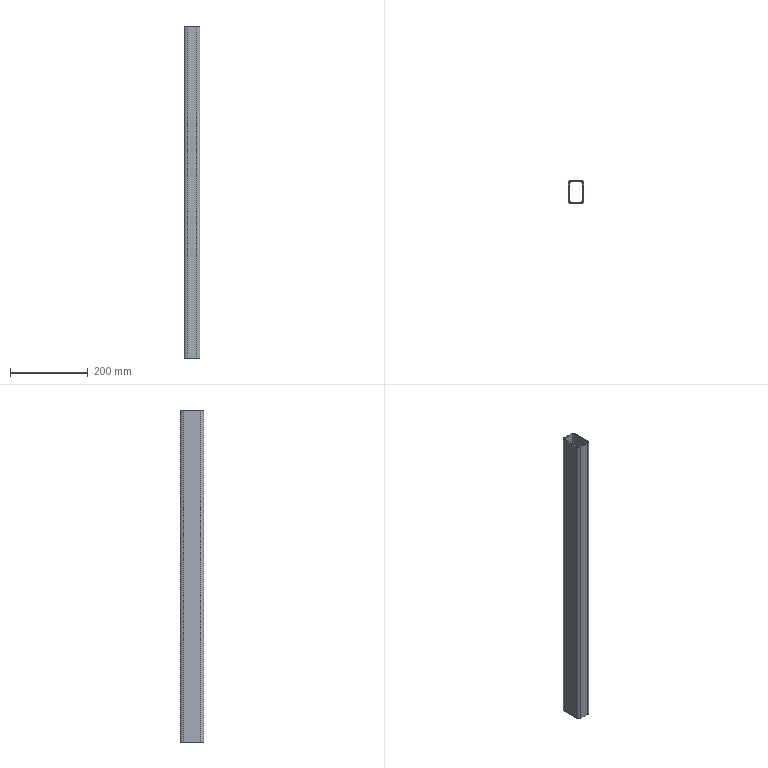Part | SolidWorks | features BaseBody 1 | 1 solid | 18 faces | box 40 x 60 x 852 mm | volume 454199 mm3 | plane 10 | cylinder 8 | commonest cylinder face diameters 9 x4 15 x4
STEP:
#1=CARTESIAN_POINT('',(17.,22.5,0.));
#2=VERTEX_POINT('',#1);
#3=CARTESIAN_POINT('',(17.,22.5,852.));
#4=VERTEX_POINT('',#3);
#5=CARTESIAN_POINT('',(17.,22.5,0.));
#6=DIRECTION('',(0.,0.,1.));
#7=VECTOR('',#6,1000.);
#8=LINE('',#5,#7);
#9=EDGE_CURVE('',#2,#4,#8,.T.);
#10=ORIENTED_EDGE('',*,*,#9,.F.);
#11=CARTESIAN_POINT('',(17.,-22.5,0.));
#12=VERTEX_POINT('',#11);
#13=CARTESIAN_POINT('',(17.,22.5,0.));
#14=DIRECTION('',(0.,1.,0.));
#15=VECTOR('',#14,1000.);
#16=LINE('',#13,#15);
#17=EDGE_CURVE('',#12,#2,#16,.T.);
#18=ORIENTED_EDGE('',*,*,#17,.F.);
#19=CARTESIAN_POINT('',(17.,-22.5,852.));
#20=VERTEX_POINT('',#19);
#21=CARTESIAN_POINT('',(17.,-22.5,0.));
#22=DIRECTION('',(0.,0.,-1.));
#23=VECTOR('',#22,1000.);
#24=LINE('',#21,#23);
#25=EDGE_CURVE('',#20,#12,#24,.T.);
#26=ORIENTED_EDGE('',*,*,#25,.F.);
#27=CARTESIAN_POINT('',(17.,22.5,852.));
#28=DIRECTION('',(0.,-1.,0.));
#29=VECTOR('',#28,1000.);
#30=LINE('',#27,#29);
#31=EDGE_CURVE('',#4,#20,#30,.T.);
#32=ORIENTED_EDGE('',*,*,#31,.F.);
#33=EDGE_LOOP('',(#10,#18,#26,#32));
#34=FACE_OUTER_BOUND('',#33,.T.);
#35=CARTESIAN_POINT('',(17.,22.5,0.));
#36=DIRECTION('',(1.,0.,0.));
#37=DIRECTION('',(0.,1.,0.));
#38=AXIS2_PLACEMENT_3D('',#35,#36,#37);
#39=PLANE('',#38);
#40=ADVANCED_FACE('',(#34),#39,.F.);
#41=CARTESIAN_POINT('',(-17.,-22.5,852.));
#42=VERTEX_POINT('',#41);
#43=CARTESIAN_POINT('',(-17.,22.5,852.));
#44=VERTEX_POINT('',#43);
#45=CARTESIAN_POINT('',(-17.,0.,852.));
#46=DIRECTION('',(0.,1.,0.));
#47=VECTOR('',#46,1000.);
#48=LINE('',#45,#47);
#49=EDGE_CURVE('',#42,#44,#48,.T.);
#50=ORIENTED_EDGE('',*,*,#49,.T.);
#51=CARTESIAN_POINT('',(-12.5,27.,852.));
#52=VERTEX_POINT('',#51);
#53=CARTESIAN_POINT('',(-12.5,22.5,852.));
#54=DIRECTION('',(0.,0.,-1.));
#55=DIRECTION('',(1.,0.,0.));
#56=AXIS2_PLACEMENT_3D('',#53,#54,#55);
#57=CIRCLE('',#56,4.5);
#58=EDGE_CURVE('',#44,#52,#57,.T.);
#59=ORIENTED_EDGE('',*,*,#58,.T.);
#60=CARTESIAN_POINT('',(12.5,27.,852.));
#61=VERTEX_POINT('',#60);
#62=CARTESIAN_POINT('',(0.,27.,852.));
#63=DIRECTION('',(1.,0.,0.));
#64=VECTOR('',#63,1000.);
#65=LINE('',#62,#64);
#66=EDGE_CURVE('',#52,#61,#65,.T.);
#67=ORIENTED_EDGE('',*,*,#66,.T.);
#68=CARTESIAN_POINT('',(12.5,22.5,852.));
#69=DIRECTION('',(0.,0.,-1.));
#70=DIRECTION('',(1.,0.,0.));
#71=AXIS2_PLACEMENT_3D('',#68,#69,#70);
#72=CIRCLE('',#71,4.5);
#73=EDGE_CURVE('',#61,#4,#72,.T.);
#74=ORIENTED_EDGE('',*,*,#73,.T.);
#75=ORIENTED_EDGE('',*,*,#31,.T.);
#76=CARTESIAN_POINT('',(12.5,-27.,852.));
#77=VERTEX_POINT('',#76);
#78=CARTESIAN_POINT('',(12.5,-22.5,852.));
#79=DIRECTION('',(0.,0.,-1.));
#80=DIRECTION('',(1.,0.,0.));
#81=AXIS2_PLACEMENT_3D('',#78,#79,#80);
#82=CIRCLE('',#81,4.5);
#83=EDGE_CURVE('',#20,#77,#82,.T.);
#84=ORIENTED_EDGE('',*,*,#83,.T.);
#85=CARTESIAN_POINT('',(-12.5,-27.,852.));
#86=VERTEX_POINT('',#85);
#87=CARTESIAN_POINT('',(0.,-27.,852.));
#88=DIRECTION('',(-1.,0.,0.));
#89=VECTOR('',#88,1000.);
#90=LINE('',#87,#89);
#91=EDGE_CURVE('',#77,#86,#90,.T.);
#92=ORIENTED_EDGE('',*,*,#91,.T.);
#93=CARTESIAN_POINT('',(-12.5,-22.5,852.));
#94=DIRECTION('',(0.,0.,-1.));
#95=DIRECTION('',(1.,0.,0.));
#96=AXIS2_PLACEMENT_3D('',#93,#94,#95);
#97=CIRCLE('',#96,4.5);
#98=EDGE_CURVE('',#86,#42,#97,.T.);
#99=ORIENTED_EDGE('',*,*,#98,.T.);
#100=EDGE_LOOP('',(#50,#59,#67,#74,#75,#84,#92,#99));
#101=FACE_BOUND('',#100,.T.);
#102=CARTESIAN_POINT('',(12.5,30.,852.));
#103=VERTEX_POINT('',#102);
#104=CARTESIAN_POINT('',(-12.5,30.,852.));
#105=VERTEX_POINT('',#104);
#106=CARTESIAN_POINT('',(0.,30.,852.));
#107=DIRECTION('',(-1.,0.,0.));
#108=VECTOR('',#107,1000.);
#109=LINE('',#106,#108);
#110=EDGE_CURVE('',#103,#105,#109,.T.);
#111=ORIENTED_EDGE('',*,*,#110,.T.);
#112=CARTESIAN_POINT('',(-20.,22.5,852.));
#113=VERTEX_POINT('',#112);
#114=CARTESIAN_POINT('',(-12.5,22.5,852.));
#115=DIRECTION('',(0.,0.,1.));
#116=DIRECTION('',(1.,0.,0.));
#117=AXIS2_PLACEMENT_3D('',#114,#115,#116);
#118=CIRCLE('',#117,7.5);
#119=EDGE_CURVE('',#105,#113,#118,.T.);
#120=ORIENTED_EDGE('',*,*,#119,.T.);
#121=CARTESIAN_POINT('',(-20.,-22.5,852.));
#122=VERTEX_POINT('',#121);
#123=CARTESIAN_POINT('',(-20.,0.,852.));
#124=DIRECTION('',(0.,-1.,0.));
#125=VECTOR('',#124,1000.);
#126=LINE('',#123,#125);
#127=EDGE_CURVE('',#113,#122,#126,.T.);
#128=ORIENTED_EDGE('',*,*,#127,.T.);
#129=CARTESIAN_POINT('',(-12.5,-30.,852.));
#130=VERTEX_POINT('',#129);
#131=CARTESIAN_POINT('',(-12.5,-22.5,852.));
#132=DIRECTION('',(0.,0.,1.));
#133=DIRECTION('',(1.,0.,0.));
#134=AXIS2_PLACEMENT_3D('',#131,#132,#133);
#135=CIRCLE('',#134,7.5);
#136=EDGE_CURVE('',#122,#130,#135,.T.);
#137=ORIENTED_EDGE('',*,*,#136,.T.);
#138=CARTESIAN_POINT('',(12.5,-30.,852.));
#139=VERTEX_POINT('',#138);
#140=CARTESIAN_POINT('',(0.,-30.,852.));
#141=DIRECTION('',(1.,0.,0.));
#142=VECTOR('',#141,1000.);
#143=LINE('',#140,#142);
#144=EDGE_CURVE('',#130,#139,#143,.T.);
#145=ORIENTED_EDGE('',*,*,#144,.T.);
#146=CARTESIAN_POINT('',(20.,-22.5,852.));
#147=VERTEX_POINT('',#146);
#148=CARTESIAN_POINT('',(12.5,-22.5,852.));
#149=DIRECTION('',(0.,0.,1.));
#150=DIRECTION('',(1.,0.,0.));
#151=AXIS2_PLACEMENT_3D('',#148,#149,#150);
#152=CIRCLE('',#151,7.5);
#153=EDGE_CURVE('',#139,#147,#152,.T.);
#154=ORIENTED_EDGE('',*,*,#153,.T.);
#155=CARTESIAN_POINT('',(20.,22.5,852.));
#156=VERTEX_POINT('',#155);
#157=CARTESIAN_POINT('',(20.,0.,852.));
#158=DIRECTION('',(0.,1.,0.));
#159=VECTOR('',#158,1000.);
#160=LINE('',#157,#159);
#161=EDGE_CURVE('',#147,#156,#160,.T.);
#162=ORIENTED_EDGE('',*,*,#161,.T.);
#163=CARTESIAN_POINT('',(12.5,22.5,852.));
#164=DIRECTION('',(0.,0.,1.));
#165=DIRECTION('',(1.,0.,0.));
#166=AXIS2_PLACEMENT_3D('',#163,#164,#165);
#167=CIRCLE('',#166,7.5);
#168=EDGE_CURVE('',#156,#103,#167,.T.);
#169=ORIENTED_EDGE('',*,*,#168,.T.);
#170=EDGE_LOOP('',(#111,#120,#128,#137,#145,#154,#162,#169));
#171=FACE_OUTER_BOUND('',#170,.T.);
#172=CARTESIAN_POINT('',(0.,0.,852.));
#173=DIRECTION('',(0.,0.,1.));
#174=DIRECTION('',(1.,0.,0.));
#175=AXIS2_PLACEMENT_3D('',#172,#173,#174);
#176=PLANE('',#175);
#177=ADVANCED_FACE('',(#101,#171),#176,.T.);
#178=CARTESIAN_POINT('',(12.5,27.,0.));
#179=VERTEX_POINT('',#178);
#180=CARTESIAN_POINT('',(12.5,27.,0.));
#181=DIRECTION('',(0.,0.,1.));
#182=VECTOR('',#181,1000.);
#183=LINE('',#180,#182);
#184=EDGE_CURVE('',#179,#61,#183,.T.);
#185=ORIENTED_EDGE('',*,*,#184,.F.);
#186=CARTESIAN_POINT('',(12.5,22.5,0.));
#187=DIRECTION('',(0.,0.,1.));
#188=DIRECTION('',(1.,0.,0.));
#189=AXIS2_PLACEMENT_3D('',#186,#187,#188);
#190=CIRCLE('',#189,4.5);
#191=EDGE_CURVE('',#2,#179,#190,.T.);
#192=ORIENTED_EDGE('',*,*,#191,.F.);
#193=ORIENTED_EDGE('',*,*,#9,.T.);
#194=ORIENTED_EDGE('',*,*,#73,.F.);
#195=EDGE_LOOP('',(#185,#192,#193,#194));
#196=FACE_OUTER_BOUND('',#195,.T.);
#197=CARTESIAN_POINT('',(12.5,22.5,0.));
#198=DIRECTION('',(0.,0.,1.));
#199=DIRECTION('',(1.,0.,0.));
#200=AXIS2_PLACEMENT_3D('',#197,#198,#199);
#201=CYLINDRICAL_SURFACE('',#200,4.5);
#202=ADVANCED_FACE('',(#196),#201,.F.);
#203=CARTESIAN_POINT('',(-17.,22.5,0.));
#204=VERTEX_POINT('',#203);
#205=CARTESIAN_POINT('',(-12.5,27.,0.));
#206=VERTEX_POINT('',#205);
#207=CARTESIAN_POINT('',(-12.5,22.5,0.));
#208=DIRECTION('',(0.,0.,-1.));
#209=DIRECTION('',(1.,0.,0.));
#210=AXIS2_PLACEMENT_3D('',#207,#208,#209);
#211=CIRCLE('',#210,4.5);
#212=EDGE_CURVE('',#204,#206,#211,.T.);
#213=ORIENTED_EDGE('',*,*,#212,.F.);
#214=CARTESIAN_POINT('',(-17.,-22.5,0.));
#215=VERTEX_POINT('',#214);
#216=CARTESIAN_POINT('',(-17.,0.,0.));
#217=DIRECTION('',(0.,1.,0.));
#218=VECTOR('',#217,1000.);
#219=LINE('',#216,#218);
#220=EDGE_CURVE('',#215,#204,#219,.T.);
#221=ORIENTED_EDGE('',*,*,#220,.F.);
#222=CARTESIAN_POINT('',(-12.5,-27.,0.));
#223=VERTEX_POINT('',#222);
#224=CARTESIAN_POINT('',(-12.5,-22.5,0.));
#225=DIRECTION('',(0.,0.,-1.));
#226=DIRECTION('',(1.,0.,0.));
#227=AXIS2_PLACEMENT_3D('',#224,#225,#226);
#228=CIRCLE('',#227,4.5);
#229=EDGE_CURVE('',#223,#215,#228,.T.);
#230=ORIENTED_EDGE('',*,*,#229,.F.);
#231=CARTESIAN_POINT('',(12.5,-27.,0.));
#232=VERTEX_POINT('',#231);
#233=CARTESIAN_POINT('',(0.,-27.,0.));
#234=DIRECTION('',(-1.,0.,0.));
#235=VECTOR('',#234,1000.);
#236=LINE('',#233,#235);
#237=EDGE_CURVE('',#232,#223,#236,.T.);
#238=ORIENTED_EDGE('',*,*,#237,.F.);
#239=CARTESIAN_POINT('',(12.5,-22.5,0.));
#240=DIRECTION('',(0.,0.,-1.));
#241=DIRECTION('',(1.,0.,0.));
#242=AXIS2_PLACEMENT_3D('',#239,#240,#241);
#243=CIRCLE('',#242,4.5);
#244=EDGE_CURVE('',#12,#232,#243,.T.);
#245=ORIENTED_EDGE('',*,*,#244,.F.);
#246=ORIENTED_EDGE('',*,*,#17,.T.);
#247=ORIENTED_EDGE('',*,*,#191,.T.);
#248=CARTESIAN_POINT('',(0.,27.,0.));
#249=DIRECTION('',(1.,0.,0.));
#250=VECTOR('',#249,1000.);
#251=LINE('',#248,#250);
#252=EDGE_CURVE('',#206,#179,#251,.T.);
#253=ORIENTED_EDGE('',*,*,#252,.F.);
#254=EDGE_LOOP('',(#213,#221,#230,#238,#245,#246,#247,#253));
#255=FACE_BOUND('',#254,.T.);
#256=CARTESIAN_POINT('',(-12.5,30.,0.));
#257=VERTEX_POINT('',#256);
#258=CARTESIAN_POINT('',(-20.,22.5,0.));
#259=VERTEX_POINT('',#258);
#260=CARTESIAN_POINT('',(-12.5,22.5,0.));
#261=DIRECTION('',(0.,0.,1.));
#262=DIRECTION('',(1.,0.,0.));
#263=AXIS2_PLACEMENT_3D('',#260,#261,#262);
#264=CIRCLE('',#263,7.5);
#265=EDGE_CURVE('',#257,#259,#264,.T.);
#266=ORIENTED_EDGE('',*,*,#265,.F.);
#267=CARTESIAN_POINT('',(12.5,30.,0.));
#268=VERTEX_POINT('',#267);
#269=CARTESIAN_POINT('',(0.,30.,0.));
#270=DIRECTION('',(-1.,0.,0.));
#271=VECTOR('',#270,1000.);
#272=LINE('',#269,#271);
#273=EDGE_CURVE('',#268,#257,#272,.T.);
#274=ORIENTED_EDGE('',*,*,#273,.F.);
#275=CARTESIAN_POINT('',(20.,22.5,0.));
#276=VERTEX_POINT('',#275);
#277=CARTESIAN_POINT('',(12.5,22.5,0.));
#278=DIRECTION('',(0.,0.,1.));
#279=DIRECTION('',(1.,0.,0.));
#280=AXIS2_PLACEMENT_3D('',#277,#278,#279);
#281=CIRCLE('',#280,7.5);
#282=EDGE_CURVE('',#276,#268,#281,.T.);
#283=ORIENTED_EDGE('',*,*,#282,.F.);
#284=CARTESIAN_POINT('',(20.,-22.5,0.));
#285=VERTEX_POINT('',#284);
#286=CARTESIAN_POINT('',(20.,0.,0.));
#287=DIRECTION('',(0.,1.,0.));
#288=VECTOR('',#287,1000.);
#289=LINE('',#286,#288);
#290=EDGE_CURVE('',#285,#276,#289,.T.);
#291=ORIENTED_EDGE('',*,*,#290,.F.);
#292=CARTESIAN_POINT('',(12.5,-30.,0.));
#293=VERTEX_POINT('',#292);
#294=CARTESIAN_POINT('',(12.5,-22.5,0.));
#295=DIRECTION('',(0.,0.,1.));
#296=DIRECTION('',(1.,0.,0.));
#297=AXIS2_PLACEMENT_3D('',#294,#295,#296);
#298=CIRCLE('',#297,7.5);
#299=EDGE_CURVE('',#293,#285,#298,.T.);
#300=ORIENTED_EDGE('',*,*,#299,.F.);
#301=CARTESIAN_POINT('',(-12.5,-30.,0.));
#302=VERTEX_POINT('',#301);
#303=CARTESIAN_POINT('',(0.,-30.,0.));
#304=DIRECTION('',(1.,0.,0.));
#305=VECTOR('',#304,1000.);
#306=LINE('',#303,#305);
#307=EDGE_CURVE('',#302,#293,#306,.T.);
#308=ORIENTED_EDGE('',*,*,#307,.F.);
#309=CARTESIAN_POINT('',(-20.,-22.5,0.));
#310=VERTEX_POINT('',#309);
#311=CARTESIAN_POINT('',(-12.5,-22.5,0.));
#312=DIRECTION('',(0.,0.,1.));
#313=DIRECTION('',(1.,0.,0.));
#314=AXIS2_PLACEMENT_3D('',#311,#312,#313);
#315=CIRCLE('',#314,7.5);
#316=EDGE_CURVE('',#310,#302,#315,.T.);
#317=ORIENTED_EDGE('',*,*,#316,.F.);
#318=CARTESIAN_POINT('',(-20.,0.,0.));
#319=DIRECTION('',(0.,-1.,0.));
#320=VECTOR('',#319,1000.);
#321=LINE('',#318,#320);
#322=EDGE_CURVE('',#259,#310,#321,.T.);
#323=ORIENTED_EDGE('',*,*,#322,.F.);
#324=EDGE_LOOP('',(#266,#274,#283,#291,#300,#308,#317,#323));
#325=FACE_OUTER_BOUND('',#324,.T.);
#326=CARTESIAN_POINT('',(0.,0.,0.));
#327=DIRECTION('',(0.,0.,1.));
#328=DIRECTION('',(1.,0.,0.));
#329=AXIS2_PLACEMENT_3D('',#326,#327,#328);
#330=PLANE('',#329);
#331=ADVANCED_FACE('',(#255,#325),#330,.F.);
#332=ORIENTED_EDGE('',*,*,#25,.T.);
#333=ORIENTED_EDGE('',*,*,#244,.T.);
#334=CARTESIAN_POINT('',(12.5,-27.,0.));
#335=DIRECTION('',(0.,0.,-1.));
#336=VECTOR('',#335,1000.);
#337=LINE('',#334,#336);
#338=EDGE_CURVE('',#77,#232,#337,.T.);
#339=ORIENTED_EDGE('',*,*,#338,.F.);
#340=ORIENTED_EDGE('',*,*,#83,.F.);
#341=EDGE_LOOP('',(#332,#333,#339,#340));
#342=FACE_OUTER_BOUND('',#341,.T.);
#343=CARTESIAN_POINT('',(12.5,-22.5,0.));
#344=DIRECTION('',(0.,0.,1.));
#345=DIRECTION('',(1.,0.,0.));
#346=AXIS2_PLACEMENT_3D('',#343,#344,#345);
#347=CYLINDRICAL_SURFACE('',#346,4.5);
#348=ADVANCED_FACE('',(#342),#347,.F.);
#349=CARTESIAN_POINT('',(-17.,22.5,0.));
#350=DIRECTION('',(0.,0.,1.));
#351=VECTOR('',#350,1000.);
#352=LINE('',#349,#351);
#353=EDGE_CURVE('',#204,#44,#352,.T.);
#354=ORIENTED_EDGE('',*,*,#353,.F.);
#355=ORIENTED_EDGE('',*,*,#212,.T.);
#356=CARTESIAN_POINT('',(-12.5,27.,0.));
#357=DIRECTION('',(0.,0.,-1.));
#358=VECTOR('',#357,1000.);
#359=LINE('',#356,#358);
#360=EDGE_CURVE('',#52,#206,#359,.T.);
#361=ORIENTED_EDGE('',*,*,#360,.F.);
#362=ORIENTED_EDGE('',*,*,#58,.F.);
#363=EDGE_LOOP('',(#354,#355,#361,#362));
#364=FACE_OUTER_BOUND('',#363,.T.);
#365=CARTESIAN_POINT('',(-12.5,22.5,0.));
#366=DIRECTION('',(0.,0.,1.));
#367=DIRECTION('',(1.,0.,0.));
#368=AXIS2_PLACEMENT_3D('',#365,#366,#367);
#369=CYLINDRICAL_SURFACE('',#368,4.5);
#370=ADVANCED_FACE('',(#364),#369,.F.);
#371=CARTESIAN_POINT('',(-17.,-22.5,0.));
#372=DIRECTION('',(0.,0.,1.));
#373=VECTOR('',#372,1000.);
#374=LINE('',#371,#373);
#375=EDGE_CURVE('',#215,#42,#374,.T.);
#376=ORIENTED_EDGE('',*,*,#375,.F.);
#377=ORIENTED_EDGE('',*,*,#220,.T.);
#378=ORIENTED_EDGE('',*,*,#353,.T.);
#379=ORIENTED_EDGE('',*,*,#49,.F.);
#380=EDGE_LOOP('',(#376,#377,#378,#379));
#381=FACE_OUTER_BOUND('',#380,.T.);
#382=CARTESIAN_POINT('',(-17.,-22.5,0.));
#383=DIRECTION('',(-1.,0.,0.));
#384=DIRECTION('',(0.,-1.,0.));
#385=AXIS2_PLACEMENT_3D('',#382,#383,#384);
#386=PLANE('',#385);
#387=ADVANCED_FACE('',(#381),#386,.F.);
#388=CARTESIAN_POINT('',(-12.5,-27.,0.));
#389=DIRECTION('',(0.,0.,1.));
#390=VECTOR('',#389,1000.);
#391=LINE('',#388,#390);
#392=EDGE_CURVE('',#223,#86,#391,.T.);
#393=ORIENTED_EDGE('',*,*,#392,.F.);
#394=ORIENTED_EDGE('',*,*,#229,.T.);
#395=ORIENTED_EDGE('',*,*,#375,.T.);
#396=ORIENTED_EDGE('',*,*,#98,.F.);
#397=EDGE_LOOP('',(#393,#394,#395,#396));
#398=FACE_OUTER_BOUND('',#397,.T.);
#399=CARTESIAN_POINT('',(-12.5,-22.5,0.));
#400=DIRECTION('',(0.,0.,1.));
#401=DIRECTION('',(1.,0.,0.));
#402=AXIS2_PLACEMENT_3D('',#399,#400,#401);
#403=CYLINDRICAL_SURFACE('',#402,4.5);
#404=ADVANCED_FACE('',(#398),#403,.F.);
#405=ORIENTED_EDGE('',*,*,#338,.T.);
#406=ORIENTED_EDGE('',*,*,#237,.T.);
#407=ORIENTED_EDGE('',*,*,#392,.T.);
#408=ORIENTED_EDGE('',*,*,#91,.F.);
#409=EDGE_LOOP('',(#405,#406,#407,#408));
#410=FACE_OUTER_BOUND('',#409,.T.);
#411=CARTESIAN_POINT('',(12.5,-27.,0.));
#412=DIRECTION('',(0.,-1.,0.));
#413=DIRECTION('',(1.,0.,0.));
#414=AXIS2_PLACEMENT_3D('',#411,#412,#413);
#415=PLANE('',#414);
#416=ADVANCED_FACE('',(#410),#415,.F.);
#417=ORIENTED_EDGE('',*,*,#360,.T.);
#418=ORIENTED_EDGE('',*,*,#252,.T.);
#419=ORIENTED_EDGE('',*,*,#184,.T.);
#420=ORIENTED_EDGE('',*,*,#66,.F.);
#421=EDGE_LOOP('',(#417,#418,#419,#420));
#422=FACE_OUTER_BOUND('',#421,.T.);
#423=CARTESIAN_POINT('',(-12.5,27.,0.));
#424=DIRECTION('',(0.,1.,0.));
#425=DIRECTION('',(-1.,0.,0.));
#426=AXIS2_PLACEMENT_3D('',#423,#424,#425);
#427=PLANE('',#426);
#428=ADVANCED_FACE('',(#422),#427,.F.);
#429=ORIENTED_EDGE('',*,*,#265,.T.);
#430=CARTESIAN_POINT('',(-20.,22.5,0.));
#431=DIRECTION('',(0.,0.,1.));
#432=VECTOR('',#431,1000.);
#433=LINE('',#430,#432);
#434=EDGE_CURVE('',#259,#113,#433,.T.);
#435=ORIENTED_EDGE('',*,*,#434,.T.);
#436=ORIENTED_EDGE('',*,*,#119,.F.);
#437=CARTESIAN_POINT('',(-12.5,30.,0.));
#438=DIRECTION('',(0.,0.,-1.));
#439=VECTOR('',#438,1000.);
#440=LINE('',#437,#439);
#441=EDGE_CURVE('',#105,#257,#440,.T.);
#442=ORIENTED_EDGE('',*,*,#441,.T.);
#443=EDGE_LOOP('',(#429,#435,#436,#442));
#444=FACE_OUTER_BOUND('',#443,.T.);
#445=CARTESIAN_POINT('',(-12.5,22.5,0.));
#446=DIRECTION('',(0.,0.,1.));
#447=DIRECTION('',(1.,0.,0.));
#448=AXIS2_PLACEMENT_3D('',#445,#446,#447);
#449=CYLINDRICAL_SURFACE('',#448,7.5);
#450=ADVANCED_FACE('',(#444),#449,.T.);
#451=ORIENTED_EDGE('',*,*,#273,.T.);
#452=ORIENTED_EDGE('',*,*,#441,.F.);
#453=ORIENTED_EDGE('',*,*,#110,.F.);
#454=CARTESIAN_POINT('',(12.5,30.,0.));
#455=DIRECTION('',(0.,0.,-1.));
#456=VECTOR('',#455,1000.);
#457=LINE('',#454,#456);
#458=EDGE_CURVE('',#103,#268,#457,.T.);
#459=ORIENTED_EDGE('',*,*,#458,.T.);
#460=EDGE_LOOP('',(#451,#452,#453,#459));
#461=FACE_OUTER_BOUND('',#460,.T.);
#462=CARTESIAN_POINT('',(-12.5,30.,0.));
#463=DIRECTION('',(0.,1.,0.));
#464=DIRECTION('',(0.,0.,1.));
#465=AXIS2_PLACEMENT_3D('',#462,#463,#464);
#466=PLANE('',#465);
#467=ADVANCED_FACE('',(#461),#466,.T.);
#468=ORIENTED_EDGE('',*,*,#282,.T.);
#469=ORIENTED_EDGE('',*,*,#458,.F.);
#470=ORIENTED_EDGE('',*,*,#168,.F.);
#471=CARTESIAN_POINT('',(20.,22.5,0.));
#472=DIRECTION('',(0.,0.,-1.));
#473=VECTOR('',#472,1000.);
#474=LINE('',#471,#473);
#475=EDGE_CURVE('',#156,#276,#474,.T.);
#476=ORIENTED_EDGE('',*,*,#475,.T.);
#477=EDGE_LOOP('',(#468,#469,#470,#476));
#478=FACE_OUTER_BOUND('',#477,.T.);
#479=CARTESIAN_POINT('',(12.5,22.5,0.));
#480=DIRECTION('',(0.,0.,1.));
#481=DIRECTION('',(1.,0.,0.));
#482=AXIS2_PLACEMENT_3D('',#479,#480,#481);
#483=CYLINDRICAL_SURFACE('',#482,7.5);
#484=ADVANCED_FACE('',(#478),#483,.T.);
#485=ORIENTED_EDGE('',*,*,#290,.T.);
#486=ORIENTED_EDGE('',*,*,#475,.F.);
#487=ORIENTED_EDGE('',*,*,#161,.F.);
#488=CARTESIAN_POINT('',(20.,-22.5,0.));
#489=DIRECTION('',(0.,0.,-1.));
#490=VECTOR('',#489,1000.);
#491=LINE('',#488,#490);
#492=EDGE_CURVE('',#147,#285,#491,.T.);
#493=ORIENTED_EDGE('',*,*,#492,.T.);
#494=EDGE_LOOP('',(#485,#486,#487,#493));
#495=FACE_OUTER_BOUND('',#494,.T.);
#496=CARTESIAN_POINT('',(20.,22.5,0.));
#497=DIRECTION('',(1.,0.,0.));
#498=DIRECTION('',(0.,0.,-1.));
#499=AXIS2_PLACEMENT_3D('',#496,#497,#498);
#500=PLANE('',#499);
#501=ADVANCED_FACE('',(#495),#500,.T.);
#502=ORIENTED_EDGE('',*,*,#299,.T.);
#503=ORIENTED_EDGE('',*,*,#492,.F.);
#504=ORIENTED_EDGE('',*,*,#153,.F.);
#505=CARTESIAN_POINT('',(12.5,-30.,0.));
#506=DIRECTION('',(0.,0.,-1.));
#507=VECTOR('',#506,1000.);
#508=LINE('',#505,#507);
#509=EDGE_CURVE('',#139,#293,#508,.T.);
#510=ORIENTED_EDGE('',*,*,#509,.T.);
#511=EDGE_LOOP('',(#502,#503,#504,#510));
#512=FACE_OUTER_BOUND('',#511,.T.);
#513=CARTESIAN_POINT('',(12.5,-22.5,0.));
#514=DIRECTION('',(0.,0.,1.));
#515=DIRECTION('',(1.,0.,0.));
#516=AXIS2_PLACEMENT_3D('',#513,#514,#515);
#517=CYLINDRICAL_SURFACE('',#516,7.5);
#518=ADVANCED_FACE('',(#512),#517,.T.);
#519=ORIENTED_EDGE('',*,*,#307,.T.);
#520=ORIENTED_EDGE('',*,*,#509,.F.);
#521=ORIENTED_EDGE('',*,*,#144,.F.);
#522=CARTESIAN_POINT('',(-12.5,-30.,0.));
#523=DIRECTION('',(0.,0.,-1.));
#524=VECTOR('',#523,1000.);
#525=LINE('',#522,#524);
#526=EDGE_CURVE('',#130,#302,#525,.T.);
#527=ORIENTED_EDGE('',*,*,#526,.T.);
#528=EDGE_LOOP('',(#519,#520,#521,#527));
#529=FACE_OUTER_BOUND('',#528,.T.);
#530=CARTESIAN_POINT('',(12.5,-30.,0.));
#531=DIRECTION('',(0.,-1.,0.));
#532=DIRECTION('',(1.,0.,0.));
#533=AXIS2_PLACEMENT_3D('',#530,#531,#532);
#534=PLANE('',#533);
#535=ADVANCED_FACE('',(#529),#534,.T.);
#536=ORIENTED_EDGE('',*,*,#316,.T.);
#537=ORIENTED_EDGE('',*,*,#526,.F.);
#538=ORIENTED_EDGE('',*,*,#136,.F.);
#539=CARTESIAN_POINT('',(-20.,-22.5,0.));
#540=DIRECTION('',(0.,0.,-1.));
#541=VECTOR('',#540,1000.);
#542=LINE('',#539,#541);
#543=EDGE_CURVE('',#122,#310,#542,.T.);
#544=ORIENTED_EDGE('',*,*,#543,.T.);
#545=EDGE_LOOP('',(#536,#537,#538,#544));
#546=FACE_OUTER_BOUND('',#545,.T.);
#547=CARTESIAN_POINT('',(-12.5,-22.5,0.));
#548=DIRECTION('',(0.,0.,1.));
#549=DIRECTION('',(1.,0.,0.));
#550=AXIS2_PLACEMENT_3D('',#547,#548,#549);
#551=CYLINDRICAL_SURFACE('',#550,7.5);
#552=ADVANCED_FACE('',(#546),#551,.T.);
#553=ORIENTED_EDGE('',*,*,#322,.T.);
#554=ORIENTED_EDGE('',*,*,#543,.F.);
#555=ORIENTED_EDGE('',*,*,#127,.F.);
#556=ORIENTED_EDGE('',*,*,#434,.F.);
#557=EDGE_LOOP('',(#553,#554,#555,#556));
#558=FACE_OUTER_BOUND('',#557,.T.);
#559=CARTESIAN_POINT('',(-20.,-22.5,0.));
#560=DIRECTION('',(-1.,0.,0.));
#561=DIRECTION('',(0.,-1.,0.));
#562=AXIS2_PLACEMENT_3D('',#559,#560,#561);
#563=PLANE('',#562);
#564=ADVANCED_FACE('',(#558),#563,.T.);
#565=CLOSED_SHELL('',(#40,#177,#202,#331,#348,#370,#387,#404,#416,#428,#450,#467,#484,#501,#518,#535,#552,#564));
#566=MANIFOLD_SOLID_BREP('',#565);
#567=CARTESIAN_POINT('',(0.,0.,0.));
#568=DIRECTION('',(0.,0.,1.));
#569=DIRECTION('',(1.,0.,0.));
#570=AXIS2_PLACEMENT_3D('',#567,#568,#569);
#571=(LENGTH_UNIT()NAMED_UNIT(*)SI_UNIT(.MILLI.,.METRE.));
#572=UNCERTAINTY_MEASURE_WITH_UNIT(LENGTH_MEASURE(0.00001),#571,'','');
#573=(NAMED_UNIT(*)PLANE_ANGLE_UNIT()SI_UNIT($,.RADIAN.));
#574=(NAMED_UNIT(*)SI_UNIT($,.STERADIAN.)SOLID_ANGLE_UNIT());
#575=(GEOMETRIC_REPRESENTATION_CONTEXT(3)GLOBAL_UNCERTAINTY_ASSIGNED_CONTEXT((#572))GLOBAL_UNIT_ASSIGNED_CONTEXT((#571,#573,#574))REPRESENTATION_CONTEXT('',''));
#576=ADVANCED_BREP_SHAPE_REPRESENTATION('',(#566,#570),#575);